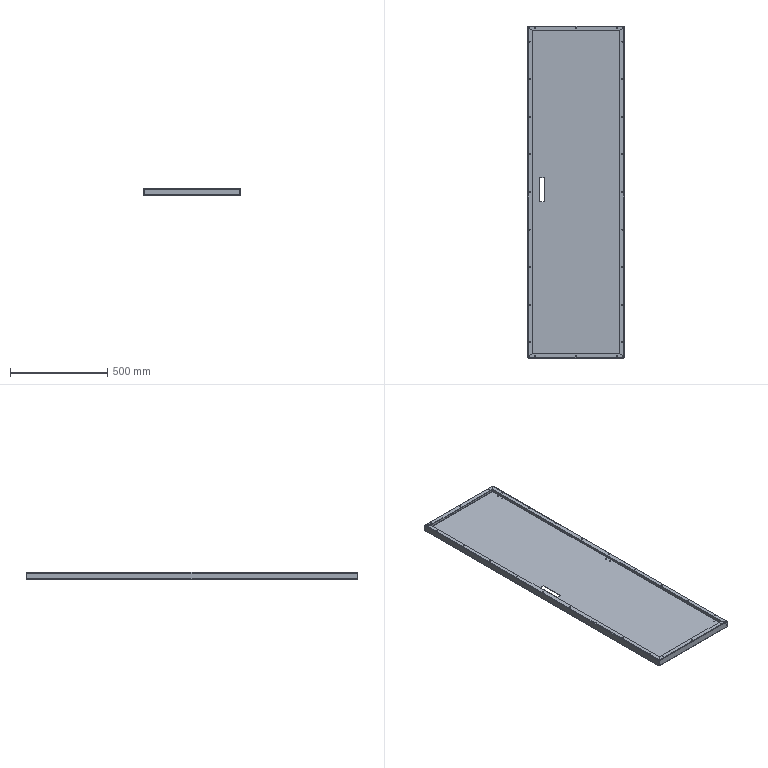Part | SolidWorks | 1 solid | 134 faces | box 494.5 x 1703 x 37 mm | volume 2668841 mm3 | cylinder 76 | plane 42 | spline 16 | commonest cylinder face diameters 5 x60 1.473 x8 6.473 x8